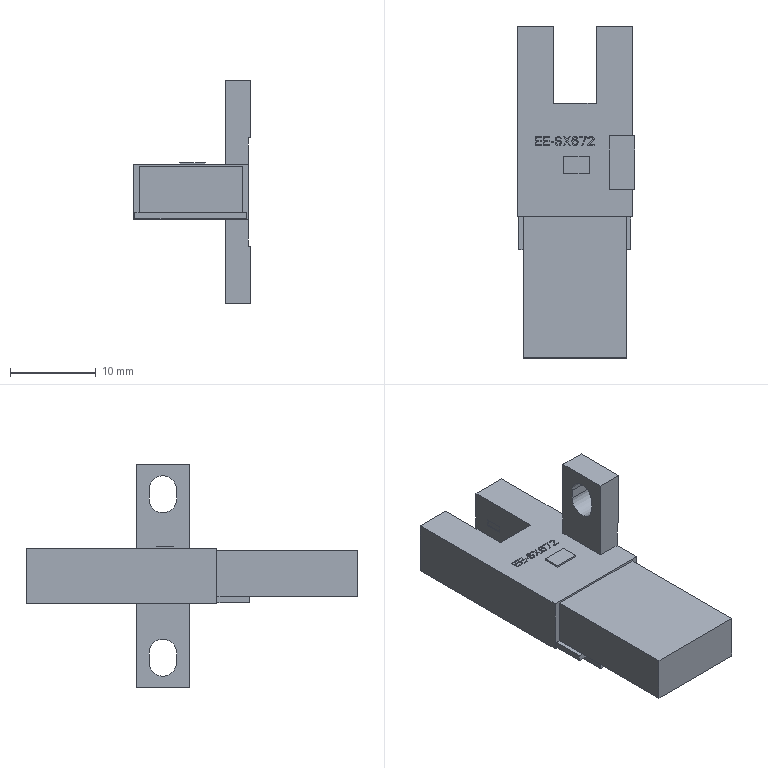Part | NX | 1 solid | 254 faces | box 13.7 x 38.6 x 26 mm | volume 2988 mm3 | plane 250 | cylinder 4 | commonest cylinder face diameters 3.2 x4